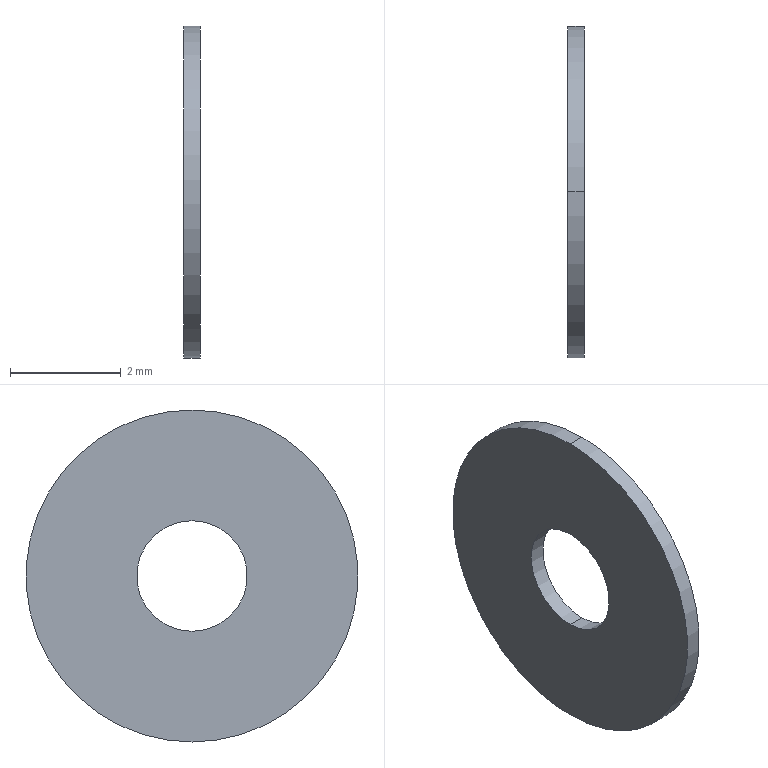Part | STEP file | 0232_Z_SCBJ2-5_3 | 1 solid | 6 faces | box 0.3 x 6 x 6 mm | volume 7.54 mm3 | cylinder 4 | plane 2 | commonest cylinder face diameters 2 x2 6 x2
STEP:
#1=CARTESIAN_POINT('',(0.,0.,0.));
#2=DIRECTION('',(0.,0.,1.));
#3=DIRECTION('',(1.,0.,0.));
#4=AXIS2_PLACEMENT_3D('',#1,#2,#3);
#5=CARTESIAN_POINT('',(0.7,0.,3.));
#6=VERTEX_POINT('',#5);
#7=CARTESIAN_POINT('',(0.7,0.,-3.));
#8=VERTEX_POINT('',#7);
#9=CARTESIAN_POINT('',(0.7,0.,0.));
#10=DIRECTION('',(-1.,0.,0.));
#11=DIRECTION('',(0.,0.,-1.));
#12=AXIS2_PLACEMENT_3D('',#9,#10,#11);
#13=CIRCLE('',#12,3.);
#14=CARTESIAN_POINT('',(0.85,0.,0.));
#15=DIRECTION('',(1.,0.,0.));
#16=DIRECTION('',(0.,0.,-1.));
#17=AXIS2_PLACEMENT_3D('',#14,#15,#16);
#18=CYLINDRICAL_SURFACE('',#17,3.);
#19=CARTESIAN_POINT('',(6.283,-0.15));
#20=DIRECTION('',(-1.,0.));
#21=VECTOR('',#20,1.);
#22=LINE('',#19,#21);
#23=(GEOMETRIC_REPRESENTATION_CONTEXT(2)PARAMETRIC_REPRESENTATION_CONTEXT()REPRESENTATION_CONTEXT('',''));
#24=DEFINITIONAL_REPRESENTATION('',(#22),#23);
#25=PCURVE('',#18,#24);
#26=CARTESIAN_POINT('',(0.7,2.,0.));
#27=DIRECTION('',(-1.,0.,0.));
#28=DIRECTION('',(0.,0.,1.));
#29=AXIS2_PLACEMENT_3D('',#26,#27,#28);
#30=PLANE('',#29);
#31=CARTESIAN_POINT('',(0.,-2.));
#32=DIRECTION('',(-1.,0.));
#33=AXIS2_PLACEMENT_2D('',#31,#32);
#34=CIRCLE('',#33,3.);
#35=(GEOMETRIC_REPRESENTATION_CONTEXT(2)PARAMETRIC_REPRESENTATION_CONTEXT()REPRESENTATION_CONTEXT('',''));
#36=DEFINITIONAL_REPRESENTATION('',(#34),#35);
#37=PCURVE('',#30,#36);
#38=SURFACE_CURVE('',#13,(#25,#37),.PCURVE_S1.);
#39=EDGE_CURVE('',#6,#8,#38,.T.);
#40=ORIENTED_EDGE('',*,*,#39,.F.);
#41=CARTESIAN_POINT('',(1.,0.,3.));
#42=VERTEX_POINT('',#41);
#43=CARTESIAN_POINT('',(0.85,0.,3.));
#44=DIRECTION('',(1.,0.,0.));
#45=VECTOR('',#44,1.);
#46=LINE('',#43,#45);
#47=CARTESIAN_POINT('',(3.142,0.));
#48=DIRECTION('',(0.,1.));
#49=VECTOR('',#48,1.);
#50=LINE('',#47,#49);
#51=(GEOMETRIC_REPRESENTATION_CONTEXT(2)PARAMETRIC_REPRESENTATION_CONTEXT()REPRESENTATION_CONTEXT('',''));
#52=DEFINITIONAL_REPRESENTATION('',(#50),#51);
#53=PCURVE('',#18,#52);
#54=CARTESIAN_POINT('',(0.85,0.,0.));
#55=DIRECTION('',(1.,0.,0.));
#56=DIRECTION('',(0.,0.,-1.));
#57=AXIS2_PLACEMENT_3D('',#54,#55,#56);
#58=CYLINDRICAL_SURFACE('',#57,3.);
#59=CARTESIAN_POINT('',(3.142,0.));
#60=DIRECTION('',(0.,1.));
#61=VECTOR('',#60,1.);
#62=LINE('',#59,#61);
#63=(GEOMETRIC_REPRESENTATION_CONTEXT(2)PARAMETRIC_REPRESENTATION_CONTEXT()REPRESENTATION_CONTEXT('',''));
#64=DEFINITIONAL_REPRESENTATION('',(#62),#63);
#65=PCURVE('',#58,#64);
#66=SURFACE_CURVE('',#46,(#53,#65),.PCURVE_S1.);
#67=EDGE_CURVE('',#6,#42,#66,.T.);
#68=ORIENTED_EDGE('',*,*,#67,.T.);
#69=CARTESIAN_POINT('',(1.,0.,-3.));
#70=VERTEX_POINT('',#69);
#71=CARTESIAN_POINT('',(1.,0.,0.));
#72=DIRECTION('',(-1.,0.,0.));
#73=DIRECTION('',(0.,0.,-1.));
#74=AXIS2_PLACEMENT_3D('',#71,#72,#73);
#75=CIRCLE('',#74,3.);
#76=CARTESIAN_POINT('',(6.283,0.15));
#77=DIRECTION('',(-1.,0.));
#78=VECTOR('',#77,1.);
#79=LINE('',#76,#78);
#80=(GEOMETRIC_REPRESENTATION_CONTEXT(2)PARAMETRIC_REPRESENTATION_CONTEXT()REPRESENTATION_CONTEXT('',''));
#81=DEFINITIONAL_REPRESENTATION('',(#79),#80);
#82=PCURVE('',#18,#81);
#83=CARTESIAN_POINT('',(1.,2.,0.));
#84=DIRECTION('',(1.,0.,0.));
#85=DIRECTION('',(0.,0.,-1.));
#86=AXIS2_PLACEMENT_3D('',#83,#84,#85);
#87=PLANE('',#86);
#88=CARTESIAN_POINT('',(3.,-2.));
#89=CARTESIAN_POINT('',(3.,-7.196));
#90=CARTESIAN_POINT('',(-1.5,-4.598));
#91=CARTESIAN_POINT('',(-6.,-2.));
#92=CARTESIAN_POINT('',(-1.5,0.5981));
#93=CARTESIAN_POINT('',(3.,3.196));
#94=CARTESIAN_POINT('',(3.,-2.));
#95=(BOUNDED_CURVE()B_SPLINE_CURVE(2,(#88,#89,#90,#91,#92,#93,#94),.UNSPECIFIED.,.T.,.F.)B_SPLINE_CURVE_WITH_KNOTS((1,2,2,2,2,1),(-2.094,0.,2.094,4.189,6.283,8.378),.UNSPECIFIED.)CURVE()GEOMETRIC_REPRESENTATION_ITEM()RATIONAL_B_SPLINE_CURVE((1.,0.5,1.,0.5,1.,0.5,1.))REPRESENTATION_ITEM(''));
#96=(GEOMETRIC_REPRESENTATION_CONTEXT(2)PARAMETRIC_REPRESENTATION_CONTEXT()REPRESENTATION_CONTEXT('',''));
#97=DEFINITIONAL_REPRESENTATION('',(#95),#96);
#98=PCURVE('',#87,#97);
#99=SURFACE_CURVE('',#75,(#82,#98),.PCURVE_S1.);
#100=EDGE_CURVE('',#42,#70,#99,.T.);
#101=ORIENTED_EDGE('',*,*,#100,.T.);
#102=CARTESIAN_POINT('',(0.85,0.,-3.));
#103=DIRECTION('',(1.,0.,0.));
#104=VECTOR('',#103,1.);
#105=LINE('',#102,#104);
#106=CARTESIAN_POINT('',(0.,0.));
#107=DIRECTION('',(0.,1.));
#108=VECTOR('',#107,1.);
#109=LINE('',#106,#108);
#110=(GEOMETRIC_REPRESENTATION_CONTEXT(2)PARAMETRIC_REPRESENTATION_CONTEXT()REPRESENTATION_CONTEXT('',''));
#111=DEFINITIONAL_REPRESENTATION('',(#109),#110);
#112=PCURVE('',#18,#111);
#113=CARTESIAN_POINT('',(6.283,0.));
#114=DIRECTION('',(0.,1.));
#115=VECTOR('',#114,1.);
#116=LINE('',#113,#115);
#117=(GEOMETRIC_REPRESENTATION_CONTEXT(2)PARAMETRIC_REPRESENTATION_CONTEXT()REPRESENTATION_CONTEXT('',''));
#118=DEFINITIONAL_REPRESENTATION('',(#116),#117);
#119=PCURVE('',#58,#118);
#120=SURFACE_CURVE('',#105,(#112,#119),.PCURVE_S1.);
#121=EDGE_CURVE('',#8,#70,#120,.T.);
#122=ORIENTED_EDGE('',*,*,#121,.F.);
#123=EDGE_LOOP('',(#40,#68,#101,#122));
#124=FACE_BOUND('',#123,.T.);
#125=ADVANCED_FACE('',(#124),#18,.T.);
#126=CARTESIAN_POINT('',(0.7,0.,-1.));
#127=VERTEX_POINT('',#126);
#128=CARTESIAN_POINT('',(1.,0.,-1.));
#129=VERTEX_POINT('',#128);
#130=CARTESIAN_POINT('',(0.85,0.,-1.));
#131=DIRECTION('',(1.,0.,0.));
#132=VECTOR('',#131,1.);
#133=LINE('',#130,#132);
#134=CARTESIAN_POINT('',(0.85,0.,0.));
#135=DIRECTION('',(1.,0.,0.));
#136=DIRECTION('',(0.,0.,-1.));
#137=AXIS2_PLACEMENT_3D('',#134,#135,#136);
#138=CYLINDRICAL_SURFACE('',#137,1.);
#139=CARTESIAN_POINT('',(6.283,0.));
#140=DIRECTION('',(0.,1.));
#141=VECTOR('',#140,1.);
#142=LINE('',#139,#141);
#143=(GEOMETRIC_REPRESENTATION_CONTEXT(2)PARAMETRIC_REPRESENTATION_CONTEXT()REPRESENTATION_CONTEXT('',''));
#144=DEFINITIONAL_REPRESENTATION('',(#142),#143);
#145=PCURVE('',#138,#144);
#146=CARTESIAN_POINT('',(0.85,0.,0.));
#147=DIRECTION('',(1.,0.,0.));
#148=DIRECTION('',(0.,0.,-1.));
#149=AXIS2_PLACEMENT_3D('',#146,#147,#148);
#150=CYLINDRICAL_SURFACE('',#149,1.);
#151=CARTESIAN_POINT('',(0.,0.));
#152=DIRECTION('',(0.,1.));
#153=VECTOR('',#152,1.);
#154=LINE('',#151,#153);
#155=(GEOMETRIC_REPRESENTATION_CONTEXT(2)PARAMETRIC_REPRESENTATION_CONTEXT()REPRESENTATION_CONTEXT('',''));
#156=DEFINITIONAL_REPRESENTATION('',(#154),#155);
#157=PCURVE('',#150,#156);
#158=SURFACE_CURVE('',#133,(#145,#157),.PCURVE_S1.);
#159=EDGE_CURVE('',#127,#129,#158,.T.);
#160=ORIENTED_EDGE('',*,*,#159,.T.);
#161=CARTESIAN_POINT('',(1.,0.,1.));
#162=VERTEX_POINT('',#161);
#163=CARTESIAN_POINT('',(1.,0.,0.));
#164=DIRECTION('',(-1.,0.,0.));
#165=DIRECTION('',(0.,0.,-1.));
#166=AXIS2_PLACEMENT_3D('',#163,#164,#165);
#167=CIRCLE('',#166,1.);
#168=CARTESIAN_POINT('',(6.283,0.15));
#169=DIRECTION('',(-1.,0.));
#170=VECTOR('',#169,1.);
#171=LINE('',#168,#170);
#172=(GEOMETRIC_REPRESENTATION_CONTEXT(2)PARAMETRIC_REPRESENTATION_CONTEXT()REPRESENTATION_CONTEXT('',''));
#173=DEFINITIONAL_REPRESENTATION('',(#171),#172);
#174=PCURVE('',#138,#173);
#175=CARTESIAN_POINT('',(1.,-2.));
#176=CARTESIAN_POINT('',(1.,-3.732));
#177=CARTESIAN_POINT('',(-0.5,-2.866));
#178=CARTESIAN_POINT('',(-2.,-2.));
#179=CARTESIAN_POINT('',(-0.5,-1.134));
#180=CARTESIAN_POINT('',(1.,-0.2679));
#181=CARTESIAN_POINT('',(1.,-2.));
#182=(BOUNDED_CURVE()B_SPLINE_CURVE(2,(#175,#176,#177,#178,#179,#180,#181),.UNSPECIFIED.,.T.,.F.)B_SPLINE_CURVE_WITH_KNOTS((1,2,2,2,2,1),(-2.094,0.,2.094,4.189,6.283,8.378),.UNSPECIFIED.)CURVE()GEOMETRIC_REPRESENTATION_ITEM()RATIONAL_B_SPLINE_CURVE((1.,0.5,1.,0.5,1.,0.5,1.))REPRESENTATION_ITEM(''));
#183=(GEOMETRIC_REPRESENTATION_CONTEXT(2)PARAMETRIC_REPRESENTATION_CONTEXT()REPRESENTATION_CONTEXT('',''));
#184=DEFINITIONAL_REPRESENTATION('',(#182),#183);
#185=PCURVE('',#87,#184);
#186=SURFACE_CURVE('',#167,(#174,#185),.PCURVE_S1.);
#187=EDGE_CURVE('',#129,#162,#186,.T.);
#188=ORIENTED_EDGE('',*,*,#187,.T.);
#189=CARTESIAN_POINT('',(0.7,0.,1.));
#190=VERTEX_POINT('',#189);
#191=CARTESIAN_POINT('',(0.85,0.,1.));
#192=DIRECTION('',(1.,0.,0.));
#193=VECTOR('',#192,1.);
#194=LINE('',#191,#193);
#195=CARTESIAN_POINT('',(3.142,0.));
#196=DIRECTION('',(0.,1.));
#197=VECTOR('',#196,1.);
#198=LINE('',#195,#197);
#199=(GEOMETRIC_REPRESENTATION_CONTEXT(2)PARAMETRIC_REPRESENTATION_CONTEXT()REPRESENTATION_CONTEXT('',''));
#200=DEFINITIONAL_REPRESENTATION('',(#198),#199);
#201=PCURVE('',#138,#200);
#202=CARTESIAN_POINT('',(3.142,0.));
#203=DIRECTION('',(0.,1.));
#204=VECTOR('',#203,1.);
#205=LINE('',#202,#204);
#206=(GEOMETRIC_REPRESENTATION_CONTEXT(2)PARAMETRIC_REPRESENTATION_CONTEXT()REPRESENTATION_CONTEXT('',''));
#207=DEFINITIONAL_REPRESENTATION('',(#205),#206);
#208=PCURVE('',#150,#207);
#209=SURFACE_CURVE('',#194,(#201,#208),.PCURVE_S1.);
#210=EDGE_CURVE('',#190,#162,#209,.T.);
#211=ORIENTED_EDGE('',*,*,#210,.F.);
#212=CARTESIAN_POINT('',(0.7,0.,0.));
#213=DIRECTION('',(1.,0.,0.));
#214=DIRECTION('',(0.,0.,-1.));
#215=AXIS2_PLACEMENT_3D('',#212,#213,#214);
#216=CIRCLE('',#215,1.);
#217=CARTESIAN_POINT('',(0.,-0.15));
#218=DIRECTION('',(1.,0.));
#219=VECTOR('',#218,1.);
#220=LINE('',#217,#219);
#221=(GEOMETRIC_REPRESENTATION_CONTEXT(2)PARAMETRIC_REPRESENTATION_CONTEXT()REPRESENTATION_CONTEXT('',''));
#222=DEFINITIONAL_REPRESENTATION('',(#220),#221);
#223=PCURVE('',#138,#222);
#224=CARTESIAN_POINT('',(-1.,-2.));
#225=CARTESIAN_POINT('',(-1.,-0.2679));
#226=CARTESIAN_POINT('',(0.5,-1.134));
#227=CARTESIAN_POINT('',(2.,-2.));
#228=CARTESIAN_POINT('',(0.5,-2.866));
#229=CARTESIAN_POINT('',(-1.,-3.732));
#230=CARTESIAN_POINT('',(-1.,-2.));
#231=(BOUNDED_CURVE()B_SPLINE_CURVE(2,(#224,#225,#226,#227,#228,#229,#230),.UNSPECIFIED.,.T.,.F.)B_SPLINE_CURVE_WITH_KNOTS((1,2,2,2,2,1),(-2.094,0.,2.094,4.189,6.283,8.378),.UNSPECIFIED.)CURVE()GEOMETRIC_REPRESENTATION_ITEM()RATIONAL_B_SPLINE_CURVE((1.,0.5,1.,0.5,1.,0.5,1.))REPRESENTATION_ITEM(''));
#232=(GEOMETRIC_REPRESENTATION_CONTEXT(2)PARAMETRIC_REPRESENTATION_CONTEXT()REPRESENTATION_CONTEXT('',''));
#233=DEFINITIONAL_REPRESENTATION('',(#231),#232);
#234=PCURVE('',#30,#233);
#235=SURFACE_CURVE('',#216,(#223,#234),.PCURVE_S1.);
#236=EDGE_CURVE('',#190,#127,#235,.T.);
#237=ORIENTED_EDGE('',*,*,#236,.T.);
#238=EDGE_LOOP('',(#160,#188,#211,#237));
#239=FACE_BOUND('',#238,.F.);
#240=ADVANCED_FACE('',(#239),#138,.F.);
#241=CARTESIAN_POINT('',(0.7,0.,0.));
#242=DIRECTION('',(-1.,0.,0.));
#243=DIRECTION('',(0.,0.,-1.));
#244=AXIS2_PLACEMENT_3D('',#241,#242,#243);
#245=CIRCLE('',#244,3.);
#246=CARTESIAN_POINT('',(0.,-2.));
#247=DIRECTION('',(-1.,0.));
#248=AXIS2_PLACEMENT_2D('',#246,#247);
#249=CIRCLE('',#248,3.);
#250=(GEOMETRIC_REPRESENTATION_CONTEXT(2)PARAMETRIC_REPRESENTATION_CONTEXT()REPRESENTATION_CONTEXT('',''));
#251=DEFINITIONAL_REPRESENTATION('',(#249),#250);
#252=PCURVE('',#30,#251);
#253=CARTESIAN_POINT('',(6.283,-0.15));
#254=DIRECTION('',(-1.,0.));
#255=VECTOR('',#254,1.);
#256=LINE('',#253,#255);
#257=(GEOMETRIC_REPRESENTATION_CONTEXT(2)PARAMETRIC_REPRESENTATION_CONTEXT()REPRESENTATION_CONTEXT('',''));
#258=DEFINITIONAL_REPRESENTATION('',(#256),#257);
#259=PCURVE('',#58,#258);
#260=SURFACE_CURVE('',#245,(#252,#259),.PCURVE_S1.);
#261=EDGE_CURVE('',#8,#6,#260,.T.);
#262=ORIENTED_EDGE('',*,*,#261,.T.);
#263=ORIENTED_EDGE('',*,*,#39,.T.);
#264=EDGE_LOOP('',(#262,#263));
#265=FACE_BOUND('',#264,.T.);
#266=CARTESIAN_POINT('',(0.7,0.,0.));
#267=DIRECTION('',(1.,0.,0.));
#268=DIRECTION('',(0.,0.,-1.));
#269=AXIS2_PLACEMENT_3D('',#266,#267,#268);
#270=CIRCLE('',#269,1.);
#271=CARTESIAN_POINT('',(-1.,-2.));
#272=CARTESIAN_POINT('',(-1.,-0.2679));
#273=CARTESIAN_POINT('',(0.5,-1.134));
#274=CARTESIAN_POINT('',(2.,-2.));
#275=CARTESIAN_POINT('',(0.5,-2.866));
#276=CARTESIAN_POINT('',(-1.,-3.732));
#277=CARTESIAN_POINT('',(-1.,-2.));
#278=(BOUNDED_CURVE()B_SPLINE_CURVE(2,(#271,#272,#273,#274,#275,#276,#277),.UNSPECIFIED.,.T.,.F.)B_SPLINE_CURVE_WITH_KNOTS((1,2,2,2,2,1),(-2.094,0.,2.094,4.189,6.283,8.378),.UNSPECIFIED.)CURVE()GEOMETRIC_REPRESENTATION_ITEM()RATIONAL_B_SPLINE_CURVE((1.,0.5,1.,0.5,1.,0.5,1.))REPRESENTATION_ITEM(''));
#279=(GEOMETRIC_REPRESENTATION_CONTEXT(2)PARAMETRIC_REPRESENTATION_CONTEXT()REPRESENTATION_CONTEXT('',''));
#280=DEFINITIONAL_REPRESENTATION('',(#278),#279);
#281=PCURVE('',#30,#280);
#282=CARTESIAN_POINT('',(0.,-0.15));
#283=DIRECTION('',(1.,0.));
#284=VECTOR('',#283,1.);
#285=LINE('',#282,#284);
#286=(GEOMETRIC_REPRESENTATION_CONTEXT(2)PARAMETRIC_REPRESENTATION_CONTEXT()REPRESENTATION_CONTEXT('',''));
#287=DEFINITIONAL_REPRESENTATION('',(#285),#286);
#288=PCURVE('',#150,#287);
#289=SURFACE_CURVE('',#270,(#281,#288),.PCURVE_S1.);
#290=EDGE_CURVE('',#127,#190,#289,.T.);
#291=ORIENTED_EDGE('',*,*,#290,.T.);
#292=ORIENTED_EDGE('',*,*,#236,.T.);
#293=EDGE_LOOP('',(#291,#292));
#294=FACE_BOUND('',#293,.T.);
#295=ADVANCED_FACE('',(#265,#294),#30,.T.);
#296=ORIENTED_EDGE('',*,*,#67,.F.);
#297=ORIENTED_EDGE('',*,*,#261,.F.);
#298=ORIENTED_EDGE('',*,*,#121,.T.);
#299=CARTESIAN_POINT('',(1.,0.,0.));
#300=DIRECTION('',(-1.,0.,0.));
#301=DIRECTION('',(0.,0.,-1.));
#302=AXIS2_PLACEMENT_3D('',#299,#300,#301);
#303=CIRCLE('',#302,3.);
#304=CARTESIAN_POINT('',(6.283,0.15));
#305=DIRECTION('',(-1.,0.));
#306=VECTOR('',#305,1.);
#307=LINE('',#304,#306);
#308=(GEOMETRIC_REPRESENTATION_CONTEXT(2)PARAMETRIC_REPRESENTATION_CONTEXT()REPRESENTATION_CONTEXT('',''));
#309=DEFINITIONAL_REPRESENTATION('',(#307),#308);
#310=PCURVE('',#58,#309);
#311=CARTESIAN_POINT('',(3.,-2.));
#312=CARTESIAN_POINT('',(3.,-7.196));
#313=CARTESIAN_POINT('',(-1.5,-4.598));
#314=CARTESIAN_POINT('',(-6.,-2.));
#315=CARTESIAN_POINT('',(-1.5,0.5981));
#316=CARTESIAN_POINT('',(3.,3.196));
#317=CARTESIAN_POINT('',(3.,-2.));
#318=(BOUNDED_CURVE()B_SPLINE_CURVE(2,(#311,#312,#313,#314,#315,#316,#317),.UNSPECIFIED.,.T.,.F.)B_SPLINE_CURVE_WITH_KNOTS((1,2,2,2,2,1),(-2.094,0.,2.094,4.189,6.283,8.378),.UNSPECIFIED.)CURVE()GEOMETRIC_REPRESENTATION_ITEM()RATIONAL_B_SPLINE_CURVE((1.,0.5,1.,0.5,1.,0.5,1.))REPRESENTATION_ITEM(''));
#319=(GEOMETRIC_REPRESENTATION_CONTEXT(2)PARAMETRIC_REPRESENTATION_CONTEXT()REPRESENTATION_CONTEXT('',''));
#320=DEFINITIONAL_REPRESENTATION('',(#318),#319);
#321=PCURVE('',#87,#320);
#322=SURFACE_CURVE('',#303,(#310,#321),.PCURVE_S1.);
#323=EDGE_CURVE('',#70,#42,#322,.T.);
#324=ORIENTED_EDGE('',*,*,#323,.T.);
#325=EDGE_LOOP('',(#296,#297,#298,#324));
#326=FACE_BOUND('',#325,.T.);
#327=ADVANCED_FACE('',(#326),#58,.T.);
#328=CARTESIAN_POINT('',(1.,0.,0.));
#329=DIRECTION('',(-1.,0.,0.));
#330=DIRECTION('',(0.,0.,-1.));
#331=AXIS2_PLACEMENT_3D('',#328,#329,#330);
#332=CIRCLE('',#331,1.);
#333=CARTESIAN_POINT('',(6.283,0.15));
#334=DIRECTION('',(-1.,0.));
#335=VECTOR('',#334,1.);
#336=LINE('',#333,#335);
#337=(GEOMETRIC_REPRESENTATION_CONTEXT(2)PARAMETRIC_REPRESENTATION_CONTEXT()REPRESENTATION_CONTEXT('',''));
#338=DEFINITIONAL_REPRESENTATION('',(#336),#337);
#339=PCURVE('',#150,#338);
#340=CARTESIAN_POINT('',(1.,-2.));
#341=CARTESIAN_POINT('',(1.,-3.732));
#342=CARTESIAN_POINT('',(-0.5,-2.866));
#343=CARTESIAN_POINT('',(-2.,-2.));
#344=CARTESIAN_POINT('',(-0.5,-1.134));
#345=CARTESIAN_POINT('',(1.,-0.2679));
#346=CARTESIAN_POINT('',(1.,-2.));
#347=(BOUNDED_CURVE()B_SPLINE_CURVE(2,(#340,#341,#342,#343,#344,#345,#346),.UNSPECIFIED.,.T.,.F.)B_SPLINE_CURVE_WITH_KNOTS((1,2,2,2,2,1),(-2.094,0.,2.094,4.189,6.283,8.378),.UNSPECIFIED.)CURVE()GEOMETRIC_REPRESENTATION_ITEM()RATIONAL_B_SPLINE_CURVE((1.,0.5,1.,0.5,1.,0.5,1.))REPRESENTATION_ITEM(''));
#348=(GEOMETRIC_REPRESENTATION_CONTEXT(2)PARAMETRIC_REPRESENTATION_CONTEXT()REPRESENTATION_CONTEXT('',''));
#349=DEFINITIONAL_REPRESENTATION('',(#347),#348);
#350=PCURVE('',#87,#349);
#351=SURFACE_CURVE('',#332,(#339,#350),.PCURVE_S1.);
#352=EDGE_CURVE('',#162,#129,#351,.T.);
#353=ORIENTED_EDGE('',*,*,#352,.T.);
#354=ORIENTED_EDGE('',*,*,#159,.F.);
#355=ORIENTED_EDGE('',*,*,#290,.T.);
#356=ORIENTED_EDGE('',*,*,#210,.T.);
#357=EDGE_LOOP('',(#353,#354,#355,#356));
#358=FACE_BOUND('',#357,.F.);
#359=ADVANCED_FACE('',(#358),#150,.F.);
#360=ORIENTED_EDGE('',*,*,#187,.T.);
#361=ORIENTED_EDGE('',*,*,#352,.T.);
#362=EDGE_LOOP('',(#360,#361));
#363=FACE_BOUND('',#362,.T.);
#364=ORIENTED_EDGE('',*,*,#323,.F.);
#365=ORIENTED_EDGE('',*,*,#100,.F.);
#366=EDGE_LOOP('',(#364,#365));
#367=FACE_BOUND('',#366,.T.);
#368=ADVANCED_FACE('',(#363,#367),#87,.T.);
#369=CLOSED_SHELL('',(#125,#240,#295,#327,#359,#368));
#370=MANIFOLD_SOLID_BREP('',#369);
#371=(LENGTH_UNIT()NAMED_UNIT(*)SI_UNIT(.MILLI.,.METRE.));
#372=UNCERTAINTY_MEASURE_WITH_UNIT(LENGTH_MEASURE(0.0000001),#371,'','');
#373=(NAMED_UNIT(*)PLANE_ANGLE_UNIT()SI_UNIT($,.RADIAN.));
#374=(NAMED_UNIT(*)SI_UNIT($,.STERADIAN.)SOLID_ANGLE_UNIT());
#375=(GEOMETRIC_REPRESENTATION_CONTEXT(3)GLOBAL_UNCERTAINTY_ASSIGNED_CONTEXT((#372))GLOBAL_UNIT_ASSIGNED_CONTEXT((#371,#373,#374))REPRESENTATION_CONTEXT('',''));
#376=ADVANCED_BREP_SHAPE_REPRESENTATION('',(#4,#370),#375);